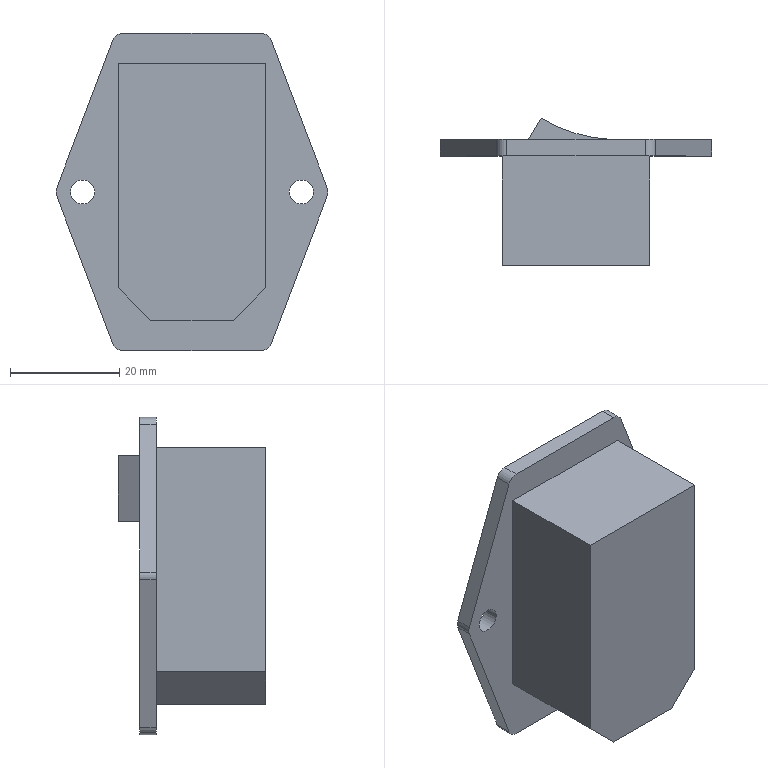Part | STEP file | DIANNAOZIDAIBAOXIANCHAZUO.stp.STEP | 1 solid | 51 faces | box 49.722 x 26.893 x 58 mm | volume 27070 mm3 | plane 40 | cylinder 11 | commonest cylinder face diameters 4 x6 4.4 x4 54.667 x1
STEP:
#1=CARTESIAN_POINT('',(7.5,0.,-23.5));
#2=VERTEX_POINT('',#1);
#3=CARTESIAN_POINT('',(-7.5,0.,-23.5));
#4=VERTEX_POINT('',#3);
#5=CARTESIAN_POINT('',(7.5,0.,-23.5));
#6=DIRECTION('',(-1.,0.,0.));
#7=VECTOR('',#6,1000.);
#8=LINE('',#5,#7);
#9=EDGE_CURVE('',#2,#4,#8,.T.);
#10=ORIENTED_EDGE('',*,*,#9,.F.);
#11=CARTESIAN_POINT('',(13.5,0.,-17.5));
#12=VERTEX_POINT('',#11);
#13=CARTESIAN_POINT('',(13.5,0.,-17.5));
#14=DIRECTION('',(-0.7071,0.,-0.7071));
#15=VECTOR('',#14,1000.);
#16=LINE('',#13,#15);
#17=EDGE_CURVE('',#12,#2,#16,.T.);
#18=ORIENTED_EDGE('',*,*,#17,.F.);
#19=CARTESIAN_POINT('',(13.5,0.,23.5));
#20=VERTEX_POINT('',#19);
#21=CARTESIAN_POINT('',(13.5,0.,23.5));
#22=DIRECTION('',(0.,0.,-1.));
#23=VECTOR('',#22,1000.);
#24=LINE('',#21,#23);
#25=EDGE_CURVE('',#20,#12,#24,.T.);
#26=ORIENTED_EDGE('',*,*,#25,.F.);
#27=CARTESIAN_POINT('',(-13.5,0.,23.5));
#28=VERTEX_POINT('',#27);
#29=CARTESIAN_POINT('',(-13.5,0.,23.5));
#30=DIRECTION('',(1.,0.,0.));
#31=VECTOR('',#30,1000.);
#32=LINE('',#29,#31);
#33=EDGE_CURVE('',#28,#20,#32,.T.);
#34=ORIENTED_EDGE('',*,*,#33,.F.);
#35=CARTESIAN_POINT('',(-13.5,0.,-17.5));
#36=VERTEX_POINT('',#35);
#37=CARTESIAN_POINT('',(-13.5,0.,-17.5));
#38=DIRECTION('',(0.,0.,1.));
#39=VECTOR('',#38,1000.);
#40=LINE('',#37,#39);
#41=EDGE_CURVE('',#36,#28,#40,.T.);
#42=ORIENTED_EDGE('',*,*,#41,.F.);
#43=CARTESIAN_POINT('',(-7.5,0.,-23.5));
#44=DIRECTION('',(-0.7071,0.,0.7071));
#45=VECTOR('',#44,1000.);
#46=LINE('',#43,#45);
#47=EDGE_CURVE('',#4,#36,#46,.T.);
#48=ORIENTED_EDGE('',*,*,#47,.F.);
#49=EDGE_LOOP('',(#10,#18,#26,#34,#42,#48));
#50=FACE_OUTER_BOUND('',#49,.T.);
#51=CARTESIAN_POINT('',(0.,0.,0.));
#52=DIRECTION('',(0.,1.,0.));
#53=DIRECTION('',(1.,0.,0.));
#54=AXIS2_PLACEMENT_3D('',#51,#52,#53);
#55=PLANE('',#54);
#56=ADVANCED_FACE('',(#50),#55,.F.);
#57=CARTESIAN_POINT('',(-7.5,20.,-23.5));
#58=VERTEX_POINT('',#57);
#59=CARTESIAN_POINT('',(-7.5,0.,-23.5));
#60=DIRECTION('',(0.,1.,0.));
#61=VECTOR('',#60,1000.);
#62=LINE('',#59,#61);
#63=EDGE_CURVE('',#4,#58,#62,.T.);
#64=ORIENTED_EDGE('',*,*,#63,.F.);
#65=ORIENTED_EDGE('',*,*,#47,.T.);
#66=CARTESIAN_POINT('',(-13.5,20.,-17.5));
#67=VERTEX_POINT('',#66);
#68=CARTESIAN_POINT('',(-13.5,0.,-17.5));
#69=DIRECTION('',(0.,1.,0.));
#70=VECTOR('',#69,1000.);
#71=LINE('',#68,#70);
#72=EDGE_CURVE('',#36,#67,#71,.T.);
#73=ORIENTED_EDGE('',*,*,#72,.T.);
#74=CARTESIAN_POINT('',(-7.5,20.,-23.5));
#75=DIRECTION('',(-0.7071,0.,0.7071));
#76=VECTOR('',#75,1000.);
#77=LINE('',#74,#76);
#78=EDGE_CURVE('',#58,#67,#77,.T.);
#79=ORIENTED_EDGE('',*,*,#78,.F.);
#80=EDGE_LOOP('',(#64,#65,#73,#79));
#81=FACE_OUTER_BOUND('',#80,.T.);
#82=CARTESIAN_POINT('',(-7.5,0.,-23.5));
#83=DIRECTION('',(-0.7071,0.,-0.7071));
#84=DIRECTION('',(-0.7071,0.,0.7071));
#85=AXIS2_PLACEMENT_3D('',#82,#83,#84);
#86=PLANE('',#85);
#87=ADVANCED_FACE('',(#81),#86,.T.);
#88=CARTESIAN_POINT('',(17.8,20.,0.));
#89=VERTEX_POINT('',#88);
#90=CARTESIAN_POINT('',(22.2,20.,0.));
#91=VERTEX_POINT('',#90);
#92=CARTESIAN_POINT('',(20.,20.,0.));
#93=DIRECTION('',(0.,1.,0.));
#94=DIRECTION('',(-1.,0.,0.));
#95=AXIS2_PLACEMENT_3D('',#92,#93,#94);
#96=CIRCLE('',#95,2.2);
#97=EDGE_CURVE('',#89,#91,#96,.T.);
#98=ORIENTED_EDGE('',*,*,#97,.T.);
#99=CARTESIAN_POINT('',(20.,20.,0.));
#100=DIRECTION('',(0.,1.,0.));
#101=DIRECTION('',(1.,0.,0.));
#102=AXIS2_PLACEMENT_3D('',#99,#100,#101);
#103=CIRCLE('',#102,2.2);
#104=EDGE_CURVE('',#91,#89,#103,.T.);
#105=ORIENTED_EDGE('',*,*,#104,.T.);
#106=EDGE_LOOP('',(#98,#105));
#107=FACE_BOUND('',#106,.T.);
#108=CARTESIAN_POINT('',(-22.2,20.,0.));
#109=VERTEX_POINT('',#108);
#110=CARTESIAN_POINT('',(-17.8,20.,0.));
#111=VERTEX_POINT('',#110);
#112=CARTESIAN_POINT('',(-20.,20.,0.));
#113=DIRECTION('',(0.,1.,0.));
#114=DIRECTION('',(-1.,0.,0.));
#115=AXIS2_PLACEMENT_3D('',#112,#113,#114);
#116=CIRCLE('',#115,2.2);
#117=EDGE_CURVE('',#109,#111,#116,.T.);
#118=ORIENTED_EDGE('',*,*,#117,.T.);
#119=CARTESIAN_POINT('',(-20.,20.,0.));
#120=DIRECTION('',(0.,1.,0.));
#121=DIRECTION('',(1.,0.,0.));
#122=AXIS2_PLACEMENT_3D('',#119,#120,#121);
#123=CIRCLE('',#122,2.2);
#124=EDGE_CURVE('',#111,#109,#123,.T.);
#125=ORIENTED_EDGE('',*,*,#124,.T.);
#126=EDGE_LOOP('',(#118,#125));
#127=FACE_BOUND('',#126,.T.);
#128=CARTESIAN_POINT('',(-13.5,20.,23.5));
#129=VERTEX_POINT('',#128);
#130=CARTESIAN_POINT('',(-13.5,20.,-17.5));
#131=DIRECTION('',(0.,0.,1.));
#132=VECTOR('',#131,1000.);
#133=LINE('',#130,#132);
#134=EDGE_CURVE('',#67,#129,#133,.T.);
#135=ORIENTED_EDGE('',*,*,#134,.T.);
#136=CARTESIAN_POINT('',(13.5,20.,23.5));
#137=VERTEX_POINT('',#136);
#138=CARTESIAN_POINT('',(-13.5,20.,23.5));
#139=DIRECTION('',(1.,0.,0.));
#140=VECTOR('',#139,1000.);
#141=LINE('',#138,#140);
#142=EDGE_CURVE('',#129,#137,#141,.T.);
#143=ORIENTED_EDGE('',*,*,#142,.T.);
#144=CARTESIAN_POINT('',(13.5,20.,-17.5));
#145=VERTEX_POINT('',#144);
#146=CARTESIAN_POINT('',(13.5,20.,23.5));
#147=DIRECTION('',(0.,0.,-1.));
#148=VECTOR('',#147,1000.);
#149=LINE('',#146,#148);
#150=EDGE_CURVE('',#137,#145,#149,.T.);
#151=ORIENTED_EDGE('',*,*,#150,.T.);
#152=CARTESIAN_POINT('',(7.5,20.,-23.5));
#153=VERTEX_POINT('',#152);
#154=CARTESIAN_POINT('',(13.5,20.,-17.5));
#155=DIRECTION('',(-0.7071,0.,-0.7071));
#156=VECTOR('',#155,1000.);
#157=LINE('',#154,#156);
#158=EDGE_CURVE('',#145,#153,#157,.T.);
#159=ORIENTED_EDGE('',*,*,#158,.T.);
#160=CARTESIAN_POINT('',(7.5,20.,-23.5));
#161=DIRECTION('',(-1.,0.,0.));
#162=VECTOR('',#161,1000.);
#163=LINE('',#160,#162);
#164=EDGE_CURVE('',#153,#58,#163,.T.);
#165=ORIENTED_EDGE('',*,*,#164,.T.);
#166=ORIENTED_EDGE('',*,*,#78,.T.);
#167=EDGE_LOOP('',(#135,#143,#151,#159,#165,#166));
#168=FACE_BOUND('',#167,.T.);
#169=CARTESIAN_POINT('',(24.731,20.,-0.7093));
#170=VERTEX_POINT('',#169);
#171=CARTESIAN_POINT('',(14.49,20.,-27.709));
#172=VERTEX_POINT('',#171);
#173=CARTESIAN_POINT('',(24.731,20.,-0.7093));
#174=DIRECTION('',(-0.3547,0.,-0.935));
#175=VECTOR('',#174,1000.);
#176=LINE('',#173,#175);
#177=EDGE_CURVE('',#170,#172,#176,.T.);
#178=ORIENTED_EDGE('',*,*,#177,.F.);
#179=CARTESIAN_POINT('',(24.731,20.,0.7093));
#180=VERTEX_POINT('',#179);
#181=CARTESIAN_POINT('',(22.861,20.,0.));
#182=DIRECTION('',(0.,-1.,0.));
#183=DIRECTION('',(0.935,0.,-0.3547));
#184=AXIS2_PLACEMENT_3D('',#181,#182,#183);
#185=CIRCLE('',#184,2.);
#186=EDGE_CURVE('',#170,#180,#185,.T.);
#187=ORIENTED_EDGE('',*,*,#186,.T.);
#188=CARTESIAN_POINT('',(14.49,20.,27.709));
#189=VERTEX_POINT('',#188);
#190=CARTESIAN_POINT('',(14.49,20.,27.709));
#191=DIRECTION('',(0.3547,0.,-0.935));
#192=VECTOR('',#191,1000.);
#193=LINE('',#190,#192);
#194=EDGE_CURVE('',#189,#180,#193,.T.);
#195=ORIENTED_EDGE('',*,*,#194,.F.);
#196=CARTESIAN_POINT('',(12.62,20.,29.));
#197=VERTEX_POINT('',#196);
#198=CARTESIAN_POINT('',(12.62,20.,27.));
#199=DIRECTION('',(0.,-1.,0.));
#200=DIRECTION('',(0.935,0.,0.3547));
#201=AXIS2_PLACEMENT_3D('',#198,#199,#200);
#202=CIRCLE('',#201,2.);
#203=EDGE_CURVE('',#189,#197,#202,.T.);
#204=ORIENTED_EDGE('',*,*,#203,.T.);
#205=CARTESIAN_POINT('',(-12.62,20.,29.));
#206=VERTEX_POINT('',#205);
#207=CARTESIAN_POINT('',(-12.62,20.,29.));
#208=DIRECTION('',(1.,0.,0.));
#209=VECTOR('',#208,1000.);
#210=LINE('',#207,#209);
#211=EDGE_CURVE('',#206,#197,#210,.T.);
#212=ORIENTED_EDGE('',*,*,#211,.F.);
#213=CARTESIAN_POINT('',(-14.49,20.,27.709));
#214=VERTEX_POINT('',#213);
#215=CARTESIAN_POINT('',(-12.62,20.,27.));
#216=DIRECTION('',(0.,-1.,0.));
#217=DIRECTION('',(0.,0.,1.));
#218=AXIS2_PLACEMENT_3D('',#215,#216,#217);
#219=CIRCLE('',#218,2.);
#220=EDGE_CURVE('',#206,#214,#219,.T.);
#221=ORIENTED_EDGE('',*,*,#220,.T.);
#222=CARTESIAN_POINT('',(-24.731,20.,0.7093));
#223=VERTEX_POINT('',#222);
#224=CARTESIAN_POINT('',(-24.731,20.,0.7093));
#225=DIRECTION('',(0.3547,0.,0.935));
#226=VECTOR('',#225,1000.);
#227=LINE('',#224,#226);
#228=EDGE_CURVE('',#223,#214,#227,.T.);
#229=ORIENTED_EDGE('',*,*,#228,.F.);
#230=CARTESIAN_POINT('',(-24.731,20.,-0.7093));
#231=VERTEX_POINT('',#230);
#232=CARTESIAN_POINT('',(-22.861,20.,0.));
#233=DIRECTION('',(0.,-1.,0.));
#234=DIRECTION('',(-0.935,0.,0.3547));
#235=AXIS2_PLACEMENT_3D('',#232,#233,#234);
#236=CIRCLE('',#235,2.);
#237=EDGE_CURVE('',#223,#231,#236,.T.);
#238=ORIENTED_EDGE('',*,*,#237,.T.);
#239=CARTESIAN_POINT('',(-14.49,20.,-27.709));
#240=VERTEX_POINT('',#239);
#241=CARTESIAN_POINT('',(-14.49,20.,-27.709));
#242=DIRECTION('',(-0.3547,0.,0.935));
#243=VECTOR('',#242,1000.);
#244=LINE('',#241,#243);
#245=EDGE_CURVE('',#240,#231,#244,.T.);
#246=ORIENTED_EDGE('',*,*,#245,.F.);
#247=CARTESIAN_POINT('',(-12.62,20.,-29.));
#248=VERTEX_POINT('',#247);
#249=CARTESIAN_POINT('',(-12.62,20.,-27.));
#250=DIRECTION('',(0.,-1.,0.));
#251=DIRECTION('',(-0.935,0.,-0.3547));
#252=AXIS2_PLACEMENT_3D('',#249,#250,#251);
#253=CIRCLE('',#252,2.);
#254=EDGE_CURVE('',#240,#248,#253,.T.);
#255=ORIENTED_EDGE('',*,*,#254,.T.);
#256=CARTESIAN_POINT('',(12.62,20.,-29.));
#257=VERTEX_POINT('',#256);
#258=CARTESIAN_POINT('',(12.62,20.,-29.));
#259=DIRECTION('',(-1.,0.,0.));
#260=VECTOR('',#259,1000.);
#261=LINE('',#258,#260);
#262=EDGE_CURVE('',#257,#248,#261,.T.);
#263=ORIENTED_EDGE('',*,*,#262,.F.);
#264=CARTESIAN_POINT('',(12.62,20.,-27.));
#265=DIRECTION('',(0.,-1.,0.));
#266=DIRECTION('',(0.,0.,-1.));
#267=AXIS2_PLACEMENT_3D('',#264,#265,#266);
#268=CIRCLE('',#267,2.);
#269=EDGE_CURVE('',#257,#172,#268,.T.);
#270=ORIENTED_EDGE('',*,*,#269,.T.);
#271=EDGE_LOOP('',(#178,#187,#195,#204,#212,#221,#229,#238,#246,#255,#263,#270));
#272=FACE_OUTER_BOUND('',#271,.T.);
#273=CARTESIAN_POINT('',(0.,20.,0.));
#274=DIRECTION('',(0.,1.,0.));
#275=DIRECTION('',(1.,0.,0.));
#276=AXIS2_PLACEMENT_3D('',#273,#274,#275);
#277=PLANE('',#276);
#278=ADVANCED_FACE('',(#107,#127,#168,#272),#277,.F.);
#279=CARTESIAN_POINT('',(7.5,0.,-23.5));
#280=DIRECTION('',(0.,1.,0.));
#281=VECTOR('',#280,1000.);
#282=LINE('',#279,#281);
#283=EDGE_CURVE('',#2,#153,#282,.T.);
#284=ORIENTED_EDGE('',*,*,#283,.F.);
#285=ORIENTED_EDGE('',*,*,#9,.T.);
#286=ORIENTED_EDGE('',*,*,#63,.T.);
#287=ORIENTED_EDGE('',*,*,#164,.F.);
#288=EDGE_LOOP('',(#284,#285,#286,#287));
#289=FACE_OUTER_BOUND('',#288,.T.);
#290=CARTESIAN_POINT('',(7.5,0.,-23.5));
#291=DIRECTION('',(0.,0.,-1.));
#292=DIRECTION('',(0.,-1.,0.));
#293=AXIS2_PLACEMENT_3D('',#290,#291,#292);
#294=PLANE('',#293);
#295=ADVANCED_FACE('',(#289),#294,.T.);
#296=CARTESIAN_POINT('',(13.5,0.,-17.5));
#297=DIRECTION('',(0.,1.,0.));
#298=VECTOR('',#297,1000.);
#299=LINE('',#296,#298);
#300=EDGE_CURVE('',#12,#145,#299,.T.);
#301=ORIENTED_EDGE('',*,*,#300,.F.);
#302=ORIENTED_EDGE('',*,*,#17,.T.);
#303=ORIENTED_EDGE('',*,*,#283,.T.);
#304=ORIENTED_EDGE('',*,*,#158,.F.);
#305=EDGE_LOOP('',(#301,#302,#303,#304));
#306=FACE_OUTER_BOUND('',#305,.T.);
#307=CARTESIAN_POINT('',(13.5,0.,-17.5));
#308=DIRECTION('',(0.7071,0.,-0.7071));
#309=DIRECTION('',(0.,-1.,0.));
#310=AXIS2_PLACEMENT_3D('',#307,#308,#309);
#311=PLANE('',#310);
#312=ADVANCED_FACE('',(#306),#311,.T.);
#313=CARTESIAN_POINT('',(13.5,0.,23.5));
#314=DIRECTION('',(0.,1.,0.));
#315=VECTOR('',#314,1000.);
#316=LINE('',#313,#315);
#317=EDGE_CURVE('',#20,#137,#316,.T.);
#318=ORIENTED_EDGE('',*,*,#317,.F.);
#319=ORIENTED_EDGE('',*,*,#25,.T.);
#320=ORIENTED_EDGE('',*,*,#300,.T.);
#321=ORIENTED_EDGE('',*,*,#150,.F.);
#322=EDGE_LOOP('',(#318,#319,#320,#321));
#323=FACE_OUTER_BOUND('',#322,.T.);
#324=CARTESIAN_POINT('',(13.5,0.,23.5));
#325=DIRECTION('',(1.,0.,0.));
#326=DIRECTION('',(0.,1.,0.));
#327=AXIS2_PLACEMENT_3D('',#324,#325,#326);
#328=PLANE('',#327);
#329=ADVANCED_FACE('',(#323),#328,.T.);
#330=CARTESIAN_POINT('',(-13.5,0.,23.5));
#331=DIRECTION('',(0.,1.,0.));
#332=VECTOR('',#331,1000.);
#333=LINE('',#330,#332);
#334=EDGE_CURVE('',#28,#129,#333,.T.);
#335=ORIENTED_EDGE('',*,*,#334,.F.);
#336=ORIENTED_EDGE('',*,*,#33,.T.);
#337=ORIENTED_EDGE('',*,*,#317,.T.);
#338=ORIENTED_EDGE('',*,*,#142,.F.);
#339=EDGE_LOOP('',(#335,#336,#337,#338));
#340=FACE_OUTER_BOUND('',#339,.T.);
#341=CARTESIAN_POINT('',(-13.5,0.,23.5));
#342=DIRECTION('',(0.,0.,1.));
#343=DIRECTION('',(1.,0.,0.));
#344=AXIS2_PLACEMENT_3D('',#341,#342,#343);
#345=PLANE('',#344);
#346=ADVANCED_FACE('',(#340),#345,.T.);
#347=ORIENTED_EDGE('',*,*,#72,.F.);
#348=ORIENTED_EDGE('',*,*,#41,.T.);
#349=ORIENTED_EDGE('',*,*,#334,.T.);
#350=ORIENTED_EDGE('',*,*,#134,.F.);
#351=EDGE_LOOP('',(#347,#348,#349,#350));
#352=FACE_OUTER_BOUND('',#351,.T.);
#353=CARTESIAN_POINT('',(-13.5,0.,-17.5));
#354=DIRECTION('',(-1.,0.,0.));
#355=DIRECTION('',(0.,0.,1.));
#356=AXIS2_PLACEMENT_3D('',#353,#354,#355);
#357=PLANE('',#356);
#358=ADVANCED_FACE('',(#352),#357,.T.);
#359=CARTESIAN_POINT('',(22.2,23.,0.));
#360=VERTEX_POINT('',#359);
#361=CARTESIAN_POINT('',(22.2,23.,0.));
#362=DIRECTION('',(0.,-1.,0.));
#363=VECTOR('',#362,1000.);
#364=LINE('',#361,#363);
#365=EDGE_CURVE('',#360,#91,#364,.T.);
#366=ORIENTED_EDGE('',*,*,#365,.F.);
#367=CARTESIAN_POINT('',(17.8,23.,0.));
#368=VERTEX_POINT('',#367);
#369=CARTESIAN_POINT('',(20.,23.,0.));
#370=DIRECTION('',(0.,1.,0.));
#371=DIRECTION('',(1.,0.,0.));
#372=AXIS2_PLACEMENT_3D('',#369,#370,#371);
#373=CIRCLE('',#372,2.2);
#374=EDGE_CURVE('',#360,#368,#373,.T.);
#375=ORIENTED_EDGE('',*,*,#374,.T.);
#376=CARTESIAN_POINT('',(17.8,23.,0.));
#377=DIRECTION('',(0.,-1.,0.));
#378=VECTOR('',#377,1000.);
#379=LINE('',#376,#378);
#380=EDGE_CURVE('',#368,#89,#379,.T.);
#381=ORIENTED_EDGE('',*,*,#380,.T.);
#382=ORIENTED_EDGE('',*,*,#104,.F.);
#383=EDGE_LOOP('',(#366,#375,#381,#382));
#384=FACE_OUTER_BOUND('',#383,.T.);
#385=CARTESIAN_POINT('',(20.,23.,0.));
#386=DIRECTION('',(0.,1.,0.));
#387=DIRECTION('',(1.,0.,0.));
#388=AXIS2_PLACEMENT_3D('',#385,#386,#387);
#389=CYLINDRICAL_SURFACE('',#388,2.2);
#390=ADVANCED_FACE('',(#384),#389,.F.);
#391=ORIENTED_EDGE('',*,*,#380,.F.);
#392=CARTESIAN_POINT('',(20.,23.,0.));
#393=DIRECTION('',(0.,1.,0.));
#394=DIRECTION('',(-1.,0.,0.));
#395=AXIS2_PLACEMENT_3D('',#392,#393,#394);
#396=CIRCLE('',#395,2.2);
#397=EDGE_CURVE('',#368,#360,#396,.T.);
#398=ORIENTED_EDGE('',*,*,#397,.T.);
#399=ORIENTED_EDGE('',*,*,#365,.T.);
#400=ORIENTED_EDGE('',*,*,#97,.F.);
#401=EDGE_LOOP('',(#391,#398,#399,#400));
#402=FACE_OUTER_BOUND('',#401,.T.);
#403=CARTESIAN_POINT('',(20.,23.,0.));
#404=DIRECTION('',(0.,1.,0.));
#405=DIRECTION('',(1.,0.,0.));
#406=AXIS2_PLACEMENT_3D('',#403,#404,#405);
#407=CYLINDRICAL_SURFACE('',#406,2.2);
#408=ADVANCED_FACE('',(#402),#407,.F.);
#409=CARTESIAN_POINT('',(-22.2,23.,0.));
#410=VERTEX_POINT('',#409);
#411=CARTESIAN_POINT('',(-17.8,23.,0.));
#412=VERTEX_POINT('',#411);
#413=CARTESIAN_POINT('',(-20.,23.,0.));
#414=DIRECTION('',(0.,1.,0.));
#415=DIRECTION('',(-1.,0.,0.));
#416=AXIS2_PLACEMENT_3D('',#413,#414,#415);
#417=CIRCLE('',#416,2.2);
#418=EDGE_CURVE('',#410,#412,#417,.T.);
#419=ORIENTED_EDGE('',*,*,#418,.F.);
#420=CARTESIAN_POINT('',(-20.,23.,0.));
#421=DIRECTION('',(0.,1.,0.));
#422=DIRECTION('',(1.,0.,0.));
#423=AXIS2_PLACEMENT_3D('',#420,#421,#422);
#424=CIRCLE('',#423,2.2);
#425=EDGE_CURVE('',#412,#410,#424,.T.);
#426=ORIENTED_EDGE('',*,*,#425,.F.);
#427=EDGE_LOOP('',(#419,#426));
#428=FACE_BOUND('',#427,.T.);
#429=ORIENTED_EDGE('',*,*,#397,.F.);
#430=ORIENTED_EDGE('',*,*,#374,.F.);
#431=EDGE_LOOP('',(#429,#430));
#432=FACE_BOUND('',#431,.T.);
#433=CARTESIAN_POINT('',(7.5,23.,-23.));
#434=VERTEX_POINT('',#433);
#435=CARTESIAN_POINT('',(-7.5,23.,-23.));
#436=VERTEX_POINT('',#435);
#437=CARTESIAN_POINT('',(7.5,23.,-23.));
#438=DIRECTION('',(-1.,0.,0.));
#439=VECTOR('',#438,1000.);
#440=LINE('',#437,#439);
#441=EDGE_CURVE('',#434,#436,#440,.T.);
#442=ORIENTED_EDGE('',*,*,#441,.F.);
#443=CARTESIAN_POINT('',(12.,23.,-18.5));
#444=VERTEX_POINT('',#443);
#445=CARTESIAN_POINT('',(12.,23.,-18.5));
#446=DIRECTION('',(-0.7071,0.,-0.7071));
#447=VECTOR('',#446,1000.);
#448=LINE('',#445,#447);
#449=EDGE_CURVE('',#444,#434,#448,.T.);
#450=ORIENTED_EDGE('',*,*,#449,.F.);
#451=CARTESIAN_POINT('',(12.,23.,-6.));
#452=VERTEX_POINT('',#451);
#453=CARTESIAN_POINT('',(12.,23.,-6.));
#454=DIRECTION('',(0.,0.,-1.));
#455=VECTOR('',#454,1000.);
#456=LINE('',#453,#455);
#457=EDGE_CURVE('',#452,#444,#456,.T.);
#458=ORIENTED_EDGE('',*,*,#457,.F.);
#459=CARTESIAN_POINT('',(-12.,23.,-6.));
#460=VERTEX_POINT('',#459);
#461=CARTESIAN_POINT('',(-12.,23.,-6.));
#462=DIRECTION('',(1.,0.,0.));
#463=VECTOR('',#462,1000.);
#464=LINE('',#461,#463);
#465=EDGE_CURVE('',#460,#452,#464,.T.);
#466=ORIENTED_EDGE('',*,*,#465,.F.);
#467=CARTESIAN_POINT('',(-12.,23.,-18.5));
#468=VERTEX_POINT('',#467);
#469=CARTESIAN_POINT('',(-12.,23.,-18.5));
#470=DIRECTION('',(0.,0.,1.));
#471=VECTOR('',#470,1000.);
#472=LINE('',#469,#471);
#473=EDGE_CURVE('',#468,#460,#472,.T.);
#474=ORIENTED_EDGE('',*,*,#473,.F.);
#475=CARTESIAN_POINT('',(-7.5,23.,-23.));
#476=DIRECTION('',(-0.7071,0.,0.7071));
#477=VECTOR('',#476,1000.);
#478=LINE('',#475,#477);
#479=EDGE_CURVE('',#436,#468,#478,.T.);
#480=ORIENTED_EDGE('',*,*,#479,.F.);
#481=EDGE_LOOP('',(#442,#450,#458,#466,#474,#480));
#482=FACE_BOUND('',#481,.T.);
#483=CARTESIAN_POINT('',(6.51,23.,10.));
#484=VERTEX_POINT('',#483);
#485=CARTESIAN_POINT('',(6.51,23.,22.));
#486=VERTEX_POINT('',#485);
#487=CARTESIAN_POINT('',(6.51,23.,10.));
#488=DIRECTION('',(0.,0.,1.));
#489=VECTOR('',#488,1000.);
#490=LINE('',#487,#489);
#491=EDGE_CURVE('',#484,#486,#490,.T.);
#492=ORIENTED_EDGE('',*,*,#491,.T.);
#493=CARTESIAN_POINT('',(-8.737,23.,22.));
#494=VERTEX_POINT('',#493);
#495=CARTESIAN_POINT('',(-8.737,23.,22.));
#496=DIRECTION('',(1.,0.,0.));
#497=VECTOR('',#496,1000.);
#498=LINE('',#495,#497);
#499=EDGE_CURVE('',#494,#486,#498,.T.);
#500=ORIENTED_EDGE('',*,*,#499,.F.);
#501=CARTESIAN_POINT('',(-8.737,23.,10.));
#502=VERTEX_POINT('',#501);
#503=CARTESIAN_POINT('',(-8.737,23.,10.));
#504=DIRECTION('',(0.,0.,1.));
#505=VECTOR('',#504,1000.);
#506=LINE('',#503,#505);
#507=EDGE_CURVE('',#502,#494,#506,.T.);
#508=ORIENTED_EDGE('',*,*,#507,.F.);
#509=CARTESIAN_POINT('',(-8.737,23.,10.));
#510=DIRECTION('',(1.,0.,0.));
#511=VECTOR('',#510,1000.);
#512=LINE('',#509,#511);
#513=EDGE_CURVE('',#502,#484,#512,.T.);
#514=ORIENTED_EDGE('',*,*,#513,.T.);
#515=EDGE_LOOP('',(#492,#500,#508,#514));
#516=FACE_BOUND('',#515,.T.);
#517=CARTESIAN_POINT('',(12.62,23.,-29.));
#518=VERTEX_POINT('',#517);
#519=CARTESIAN_POINT('',(-12.62,23.,-29.));
#520=VERTEX_POINT('',#519);
#521=CARTESIAN_POINT('',(12.62,23.,-29.));
#522=DIRECTION('',(-1.,0.,0.));
#523=VECTOR('',#522,1000.);
#524=LINE('',#521,#523);
#525=EDGE_CURVE('',#518,#520,#524,.T.);
#526=ORIENTED_EDGE('',*,*,#525,.T.);
#527=CARTESIAN_POINT('',(-14.49,23.,-27.709));
#528=VERTEX_POINT('',#527);
#529=CARTESIAN_POINT('',(-12.62,23.,-27.));
#530=DIRECTION('',(0.,1.,0.));
#531=DIRECTION('',(0.,0.,-1.));
#532=AXIS2_PLACEMENT_3D('',#529,#530,#531);
#533=CIRCLE('',#532,2.);
#534=EDGE_CURVE('',#520,#528,#533,.T.);
#535=ORIENTED_EDGE('',*,*,#534,.T.);
#536=CARTESIAN_POINT('',(-24.731,23.,-0.7093));
#537=VERTEX_POINT('',#536);
#538=CARTESIAN_POINT('',(-14.49,23.,-27.709));
#539=DIRECTION('',(-0.3547,0.,0.935));
#540=VECTOR('',#539,1000.);
#541=LINE('',#538,#540);
#542=EDGE_CURVE('',#528,#537,#541,.T.);
#543=ORIENTED_EDGE('',*,*,#542,.T.);
#544=CARTESIAN_POINT('',(-24.731,23.,0.7093));
#545=VERTEX_POINT('',#544);
#546=CARTESIAN_POINT('',(-22.861,23.,0.));
#547=DIRECTION('',(0.,1.,0.));
#548=DIRECTION('',(-0.935,0.,-0.3547));
#549=AXIS2_PLACEMENT_3D('',#546,#547,#548);
#550=CIRCLE('',#549,2.);
#551=EDGE_CURVE('',#537,#545,#550,.T.);
#552=ORIENTED_EDGE('',*,*,#551,.T.);
#553=CARTESIAN_POINT('',(-14.49,23.,27.709));
#554=VERTEX_POINT('',#553);
#555=CARTESIAN_POINT('',(-24.731,23.,0.7093));
#556=DIRECTION('',(0.3547,0.,0.935));
#557=VECTOR('',#556,1000.);
#558=LINE('',#555,#557);
#559=EDGE_CURVE('',#545,#554,#558,.T.);
#560=ORIENTED_EDGE('',*,*,#559,.T.);
#561=CARTESIAN_POINT('',(-12.62,23.,29.));
#562=VERTEX_POINT('',#561);
#563=CARTESIAN_POINT('',(-12.62,23.,27.));
#564=DIRECTION('',(0.,1.,0.));
#565=DIRECTION('',(-0.935,0.,0.3547));
#566=AXIS2_PLACEMENT_3D('',#563,#564,#565);
#567=CIRCLE('',#566,2.);
#568=EDGE_CURVE('',#554,#562,#567,.T.);
#569=ORIENTED_EDGE('',*,*,#568,.T.);
#570=CARTESIAN_POINT('',(12.62,23.,29.));
#571=VERTEX_POINT('',#570);
#572=CARTESIAN_POINT('',(-12.62,23.,29.));
#573=DIRECTION('',(1.,0.,0.));
#574=VECTOR('',#573,1000.);
#575=LINE('',#572,#574);
#576=EDGE_CURVE('',#562,#571,#575,.T.);
#577=ORIENTED_EDGE('',*,*,#576,.T.);
#578=CARTESIAN_POINT('',(14.49,23.,27.709));
#579=VERTEX_POINT('',#578);
#580=CARTESIAN_POINT('',(12.62,23.,27.));
#581=DIRECTION('',(0.,1.,0.));
#582=DIRECTION('',(0.,0.,1.));
#583=AXIS2_PLACEMENT_3D('',#580,#581,#582);
#584=CIRCLE('',#583,2.);
#585=EDGE_CURVE('',#571,#579,#584,.T.);
#586=ORIENTED_EDGE('',*,*,#585,.T.);
#587=CARTESIAN_POINT('',(24.731,23.,0.7093));
#588=VERTEX_POINT('',#587);
#589=CARTESIAN_POINT('',(14.49,23.,27.709));
#590=DIRECTION('',(0.3547,0.,-0.935));
#591=VECTOR('',#590,1000.);
#592=LINE('',#589,#591);
#593=EDGE_CURVE('',#579,#588,#592,.T.);
#594=ORIENTED_EDGE('',*,*,#593,.T.);
#595=CARTESIAN_POINT('',(24.731,23.,-0.7093));
#596=VERTEX_POINT('',#595);
#597=CARTESIAN_POINT('',(22.861,23.,0.));
#598=DIRECTION('',(0.,1.,0.));
#599=DIRECTION('',(0.935,0.,0.3547));
#600=AXIS2_PLACEMENT_3D('',#597,#598,#599);
#601=CIRCLE('',#600,2.);
#602=EDGE_CURVE('',#588,#596,#601,.T.);
#603=ORIENTED_EDGE('',*,*,#602,.T.);
#604=CARTESIAN_POINT('',(14.49,23.,-27.709));
#605=VERTEX_POINT('',#604);
#606=CARTESIAN_POINT('',(24.731,23.,-0.7093));
#607=DIRECTION('',(-0.3547,0.,-0.935));
#608=VECTOR('',#607,1000.);
#609=LINE('',#606,#608);
#610=EDGE_CURVE('',#596,#605,#609,.T.);
#611=ORIENTED_EDGE('',*,*,#610,.T.);
#612=CARTESIAN_POINT('',(12.62,23.,-27.));
#613=DIRECTION('',(0.,1.,0.));
#614=DIRECTION('',(0.935,0.,-0.3547));
#615=AXIS2_PLACEMENT_3D('',#612,#613,#614);
#616=CIRCLE('',#615,2.);
#617=EDGE_CURVE('',#605,#518,#616,.T.);
#618=ORIENTED_EDGE('',*,*,#617,.T.);
#619=EDGE_LOOP('',(#526,#535,#543,#552,#560,#569,#577,#586,#594,#603,#611,#618));
#620=FACE_OUTER_BOUND('',#619,.T.);
#621=CARTESIAN_POINT('',(0.,23.,0.));
#622=DIRECTION('',(0.,1.,0.));
#623=DIRECTION('',(1.,0.,0.));
#624=AXIS2_PLACEMENT_3D('',#621,#622,#623);
#625=PLANE('',#624);
#626=ADVANCED_FACE('',(#428,#432,#482,#516,#620),#625,.T.);
#627=CARTESIAN_POINT('',(-17.8,23.,0.));
#628=DIRECTION('',(0.,-1.,0.));
#629=VECTOR('',#628,1000.);
#630=LINE('',#627,#629);
#631=EDGE_CURVE('',#412,#111,#630,.T.);
#632=ORIENTED_EDGE('',*,*,#631,.F.);
#633=ORIENTED_EDGE('',*,*,#425,.T.);
#634=CARTESIAN_POINT('',(-22.2,23.,0.));
#635=DIRECTION('',(0.,-1.,0.));
#636=VECTOR('',#635,1000.);
#637=LINE('',#634,#636);
#638=EDGE_CURVE('',#410,#109,#637,.T.);
#639=ORIENTED_EDGE('',*,*,#638,.T.);
#640=ORIENTED_EDGE('',*,*,#124,.F.);
#641=EDGE_LOOP('',(#632,#633,#639,#640));
#642=FACE_OUTER_BOUND('',#641,.T.);
#643=CARTESIAN_POINT('',(-20.,23.,0.));
#644=DIRECTION('',(0.,1.,0.));
#645=DIRECTION('',(1.,0.,0.));
#646=AXIS2_PLACEMENT_3D('',#643,#644,#645);
#647=CYLINDRICAL_SURFACE('',#646,2.2);
#648=ADVANCED_FACE('',(#642),#647,.F.);
#649=ORIENTED_EDGE('',*,*,#638,.F.);
#650=ORIENTED_EDGE('',*,*,#418,.T.);
#651=ORIENTED_EDGE('',*,*,#631,.T.);
#652=ORIENTED_EDGE('',*,*,#117,.F.);
#653=EDGE_LOOP('',(#649,#650,#651,#652));
#654=FACE_OUTER_BOUND('',#653,.T.);
#655=CARTESIAN_POINT('',(-20.,23.,0.));
#656=DIRECTION('',(0.,1.,0.));
#657=DIRECTION('',(1.,0.,0.));
#658=AXIS2_PLACEMENT_3D('',#655,#656,#657);
#659=CYLINDRICAL_SURFACE('',#658,2.2);
#660=ADVANCED_FACE('',(#654),#659,.F.);
#661=CARTESIAN_POINT('',(12.62,23.,-29.));
#662=DIRECTION('',(0.,-1.,0.));
#663=VECTOR('',#662,1000.);
#664=LINE('',#661,#663);
#665=EDGE_CURVE('',#518,#257,#664,.T.);
#666=ORIENTED_EDGE('',*,*,#665,.F.);
#667=ORIENTED_EDGE('',*,*,#617,.F.);
#668=CARTESIAN_POINT('',(14.49,23.,-27.709));
#669=DIRECTION('',(0.,-1.,0.));
#670=VECTOR('',#669,1000.);
#671=LINE('',#668,#670);
#672=EDGE_CURVE('',#605,#172,#671,.T.);
#673=ORIENTED_EDGE('',*,*,#672,.T.);
#674=ORIENTED_EDGE('',*,*,#269,.F.);
#675=EDGE_LOOP('',(#666,#667,#673,#674));
#676=FACE_OUTER_BOUND('',#675,.T.);
#677=CARTESIAN_POINT('',(12.62,52.983,-27.));
#678=DIRECTION('',(0.,-1.,0.));
#679=DIRECTION('',(0.,0.,-1.));
#680=AXIS2_PLACEMENT_3D('',#677,#678,#679);
#681=CYLINDRICAL_SURFACE('',#680,2.);
#682=ADVANCED_FACE('',(#676),#681,.T.);
#683=ORIENTED_EDGE('',*,*,#610,.F.);
#684=CARTESIAN_POINT('',(24.731,23.,-0.7093));
#685=DIRECTION('',(0.,-1.,0.));
#686=VECTOR('',#685,1000.);
#687=LINE('',#684,#686);
#688=EDGE_CURVE('',#596,#170,#687,.T.);
#689=ORIENTED_EDGE('',*,*,#688,.T.);
#690=ORIENTED_EDGE('',*,*,#177,.T.);
#691=ORIENTED_EDGE('',*,*,#672,.F.);
#692=EDGE_LOOP('',(#683,#689,#690,#691));
#693=FACE_OUTER_BOUND('',#692,.T.);
#694=CARTESIAN_POINT('',(25.,20.,0.));
#695=DIRECTION('',(0.935,0.,-0.3547));
#696=DIRECTION('',(0.,-1.,0.));
#697=AXIS2_PLACEMENT_3D('',#694,#695,#696);
#698=PLANE('',#697);
#699=ADVANCED_FACE('',(#693),#698,.T.);
#700=ORIENTED_EDGE('',*,*,#688,.F.);
#701=ORIENTED_EDGE('',*,*,#602,.F.);
#702=CARTESIAN_POINT('',(24.731,23.,0.7093));
#703=DIRECTION('',(0.,-1.,0.));
#704=VECTOR('',#703,1000.);
#705=LINE('',#702,#704);
#706=EDGE_CURVE('',#588,#180,#705,.T.);
#707=ORIENTED_EDGE('',*,*,#706,.T.);
#708=ORIENTED_EDGE('',*,*,#186,.F.);
#709=EDGE_LOOP('',(#700,#701,#707,#708));
#710=FACE_OUTER_BOUND('',#709,.T.);
#711=CARTESIAN_POINT('',(22.861,52.983,0.));
#712=DIRECTION('',(0.,-1.,0.));
#713=DIRECTION('',(0.935,0.,-0.3547));
#714=AXIS2_PLACEMENT_3D('',#711,#712,#713);
#715=CYLINDRICAL_SURFACE('',#714,2.);
#716=ADVANCED_FACE('',(#710),#715,.T.);
#717=ORIENTED_EDGE('',*,*,#194,.T.);
#718=ORIENTED_EDGE('',*,*,#706,.F.);
#719=ORIENTED_EDGE('',*,*,#593,.F.);
#720=CARTESIAN_POINT('',(14.49,23.,27.709));
#721=DIRECTION('',(0.,-1.,0.));
#722=VECTOR('',#721,1000.);
#723=LINE('',#720,#722);
#724=EDGE_CURVE('',#579,#189,#723,.T.);
#725=ORIENTED_EDGE('',*,*,#724,.T.);
#726=EDGE_LOOP('',(#717,#718,#719,#725));
#727=FACE_OUTER_BOUND('',#726,.T.);
#728=CARTESIAN_POINT('',(14.,20.,29.));
#729=DIRECTION('',(0.935,0.,0.3547));
#730=DIRECTION('',(0.,-1.,0.));
#731=AXIS2_PLACEMENT_3D('',#728,#729,#730);
#732=PLANE('',#731);
#733=ADVANCED_FACE('',(#727),#732,.T.);
#734=ORIENTED_EDGE('',*,*,#724,.F.);
#735=ORIENTED_EDGE('',*,*,#585,.F.);
#736=CARTESIAN_POINT('',(12.62,23.,29.));
#737=DIRECTION('',(0.,-1.,0.));
#738=VECTOR('',#737,1000.);
#739=LINE('',#736,#738);
#740=EDGE_CURVE('',#571,#197,#739,.T.);
#741=ORIENTED_EDGE('',*,*,#740,.T.);
#742=ORIENTED_EDGE('',*,*,#203,.F.);
#743=EDGE_LOOP('',(#734,#735,#741,#742));
#744=FACE_OUTER_BOUND('',#743,.T.);
#745=CARTESIAN_POINT('',(12.62,52.983,27.));
#746=DIRECTION('',(0.,-1.,0.));
#747=DIRECTION('',(0.935,0.,0.3547));
#748=AXIS2_PLACEMENT_3D('',#745,#746,#747);
#749=CYLINDRICAL_SURFACE('',#748,2.);
#750=ADVANCED_FACE('',(#744),#749,.T.);
#751=ORIENTED_EDGE('',*,*,#211,.T.);
#752=ORIENTED_EDGE('',*,*,#740,.F.);
#753=ORIENTED_EDGE('',*,*,#576,.F.);
#754=CARTESIAN_POINT('',(-12.62,23.,29.));
#755=DIRECTION('',(0.,-1.,0.));
#756=VECTOR('',#755,1000.);
#757=LINE('',#754,#756);
#758=EDGE_CURVE('',#562,#206,#757,.T.);
#759=ORIENTED_EDGE('',*,*,#758,.T.);
#760=EDGE_LOOP('',(#751,#752,#753,#759));
#761=FACE_OUTER_BOUND('',#760,.T.);
#762=CARTESIAN_POINT('',(-14.,20.,29.));
#763=DIRECTION('',(0.,0.,1.));
#764=DIRECTION('',(1.,0.,0.));
#765=AXIS2_PLACEMENT_3D('',#762,#763,#764);
#766=PLANE('',#765);
#767=ADVANCED_FACE('',(#761),#766,.T.);
#768=ORIENTED_EDGE('',*,*,#758,.F.);
#769=ORIENTED_EDGE('',*,*,#568,.F.);
#770=CARTESIAN_POINT('',(-14.49,23.,27.709));
#771=DIRECTION('',(0.,-1.,0.));
#772=VECTOR('',#771,1000.);
#773=LINE('',#770,#772);
#774=EDGE_CURVE('',#554,#214,#773,.T.);
#775=ORIENTED_EDGE('',*,*,#774,.T.);
#776=ORIENTED_EDGE('',*,*,#220,.F.);
#777=EDGE_LOOP('',(#768,#769,#775,#776));
#778=FACE_OUTER_BOUND('',#777,.T.);
#779=CARTESIAN_POINT('',(-12.62,52.983,27.));
#780=DIRECTION('',(0.,-1.,0.));
#781=DIRECTION('',(0.,0.,1.));
#782=AXIS2_PLACEMENT_3D('',#779,#780,#781);
#783=CYLINDRICAL_SURFACE('',#782,2.);
#784=ADVANCED_FACE('',(#778),#783,.T.);
#785=ORIENTED_EDGE('',*,*,#228,.T.);
#786=ORIENTED_EDGE('',*,*,#774,.F.);
#787=ORIENTED_EDGE('',*,*,#559,.F.);
#788=CARTESIAN_POINT('',(-24.731,23.,0.7093));
#789=DIRECTION('',(0.,-1.,0.));
#790=VECTOR('',#789,1000.);
#791=LINE('',#788,#790);
#792=EDGE_CURVE('',#545,#223,#791,.T.);
#793=ORIENTED_EDGE('',*,*,#792,.T.);
#794=EDGE_LOOP('',(#785,#786,#787,#793));
#795=FACE_OUTER_BOUND('',#794,.T.);
#796=CARTESIAN_POINT('',(-25.,20.,0.));
#797=DIRECTION('',(-0.935,0.,0.3547));
#798=DIRECTION('',(0.,1.,0.));
#799=AXIS2_PLACEMENT_3D('',#796,#797,#798);
#800=PLANE('',#799);
#801=ADVANCED_FACE('',(#795),#800,.T.);
#802=ORIENTED_EDGE('',*,*,#792,.F.);
#803=ORIENTED_EDGE('',*,*,#551,.F.);
#804=CARTESIAN_POINT('',(-24.731,23.,-0.7093));
#805=DIRECTION('',(0.,-1.,0.));
#806=VECTOR('',#805,1000.);
#807=LINE('',#804,#806);
#808=EDGE_CURVE('',#537,#231,#807,.T.);
#809=ORIENTED_EDGE('',*,*,#808,.T.);
#810=ORIENTED_EDGE('',*,*,#237,.F.);
#811=EDGE_LOOP('',(#802,#803,#809,#810));
#812=FACE_OUTER_BOUND('',#811,.T.);
#813=CARTESIAN_POINT('',(-22.861,52.983,0.));
#814=DIRECTION('',(0.,-1.,0.));
#815=DIRECTION('',(-0.935,0.,0.3547));
#816=AXIS2_PLACEMENT_3D('',#813,#814,#815);
#817=CYLINDRICAL_SURFACE('',#816,2.);
#818=ADVANCED_FACE('',(#812),#817,.T.);
#819=ORIENTED_EDGE('',*,*,#245,.T.);
#820=ORIENTED_EDGE('',*,*,#808,.F.);
#821=ORIENTED_EDGE('',*,*,#542,.F.);
#822=CARTESIAN_POINT('',(-14.49,23.,-27.709));
#823=DIRECTION('',(0.,-1.,0.));
#824=VECTOR('',#823,1000.);
#825=LINE('',#822,#824);
#826=EDGE_CURVE('',#528,#240,#825,.T.);
#827=ORIENTED_EDGE('',*,*,#826,.T.);
#828=EDGE_LOOP('',(#819,#820,#821,#827));
#829=FACE_OUTER_BOUND('',#828,.T.);
#830=CARTESIAN_POINT('',(-14.,20.,-29.));
#831=DIRECTION('',(-0.935,0.,-0.3547));
#832=DIRECTION('',(-0.3547,0.,0.935));
#833=AXIS2_PLACEMENT_3D('',#830,#831,#832);
#834=PLANE('',#833);
#835=ADVANCED_FACE('',(#829),#834,.T.);
#836=ORIENTED_EDGE('',*,*,#826,.F.);
#837=ORIENTED_EDGE('',*,*,#534,.F.);
#838=CARTESIAN_POINT('',(-12.62,23.,-29.));
#839=DIRECTION('',(0.,-1.,0.));
#840=VECTOR('',#839,1000.);
#841=LINE('',#838,#840);
#842=EDGE_CURVE('',#520,#248,#841,.T.);
#843=ORIENTED_EDGE('',*,*,#842,.T.);
#844=ORIENTED_EDGE('',*,*,#254,.F.);
#845=EDGE_LOOP('',(#836,#837,#843,#844));
#846=FACE_OUTER_BOUND('',#845,.T.);
#847=CARTESIAN_POINT('',(-12.62,52.983,-27.));
#848=DIRECTION('',(0.,-1.,0.));
#849=DIRECTION('',(-0.935,0.,-0.3547));
#850=AXIS2_PLACEMENT_3D('',#847,#848,#849);
#851=CYLINDRICAL_SURFACE('',#850,2.);
#852=ADVANCED_FACE('',(#846),#851,.T.);
#853=ORIENTED_EDGE('',*,*,#262,.T.);
#854=ORIENTED_EDGE('',*,*,#842,.F.);
#855=ORIENTED_EDGE('',*,*,#525,.F.);
#856=ORIENTED_EDGE('',*,*,#665,.T.);
#857=EDGE_LOOP('',(#853,#854,#855,#856));
#858=FACE_OUTER_BOUND('',#857,.T.);
#859=CARTESIAN_POINT('',(14.,20.,-29.));
#860=DIRECTION('',(0.,0.,-1.));
#861=DIRECTION('',(0.,-1.,0.));
#862=AXIS2_PLACEMENT_3D('',#859,#860,#861);
#863=PLANE('',#862);
#864=ADVANCED_FACE('',(#858),#863,.T.);
#865=CARTESIAN_POINT('',(-12.,11.,-18.5));
#866=VERTEX_POINT('',#865);
#867=CARTESIAN_POINT('',(-12.,23.,-18.5));
#868=DIRECTION('',(0.,-1.,0.));
#869=VECTOR('',#868,1000.);
#870=LINE('',#867,#869);
#871=EDGE_CURVE('',#468,#866,#870,.T.);
#872=ORIENTED_EDGE('',*,*,#871,.T.);
#873=CARTESIAN_POINT('',(-7.5,11.,-23.));
#874=VERTEX_POINT('',#873);
#875=CARTESIAN_POINT('',(-7.5,11.,-23.));
#876=DIRECTION('',(-0.7071,0.,0.7071));
#877=VECTOR('',#876,1000.);
#878=LINE('',#875,#877);
#879=EDGE_CURVE('',#874,#866,#878,.T.);
#880=ORIENTED_EDGE('',*,*,#879,.F.);
#881=CARTESIAN_POINT('',(-7.5,23.,-23.));
#882=DIRECTION('',(0.,-1.,0.));
#883=VECTOR('',#882,1000.);
#884=LINE('',#881,#883);
#885=EDGE_CURVE('',#436,#874,#884,.T.);
#886=ORIENTED_EDGE('',*,*,#885,.F.);
#887=ORIENTED_EDGE('',*,*,#479,.T.);
#888=EDGE_LOOP('',(#872,#880,#886,#887));
#889=FACE_OUTER_BOUND('',#888,.T.);
#890=CARTESIAN_POINT('',(-7.5,23.,-23.));
#891=DIRECTION('',(-0.7071,0.,-0.7071));
#892=DIRECTION('',(-0.7071,0.,0.7071));
#893=AXIS2_PLACEMENT_3D('',#890,#891,#892);
#894=PLANE('',#893);
#895=ADVANCED_FACE('',(#889),#894,.F.);
#896=ORIENTED_EDGE('',*,*,#885,.T.);
#897=CARTESIAN_POINT('',(7.5,11.,-23.));
#898=VERTEX_POINT('',#897);
#899=CARTESIAN_POINT('',(7.5,11.,-23.));
#900=DIRECTION('',(-1.,0.,0.));
#901=VECTOR('',#900,1000.);
#902=LINE('',#899,#901);
#903=EDGE_CURVE('',#898,#874,#902,.T.);
#904=ORIENTED_EDGE('',*,*,#903,.F.);
#905=CARTESIAN_POINT('',(7.5,23.,-23.));
#906=DIRECTION('',(0.,-1.,0.));
#907=VECTOR('',#906,1000.);
#908=LINE('',#905,#907);
#909=EDGE_CURVE('',#434,#898,#908,.T.);
#910=ORIENTED_EDGE('',*,*,#909,.F.);
#911=ORIENTED_EDGE('',*,*,#441,.T.);
#912=EDGE_LOOP('',(#896,#904,#910,#911));
#913=FACE_OUTER_BOUND('',#912,.T.);
#914=CARTESIAN_POINT('',(7.5,23.,-23.));
#915=DIRECTION('',(0.,0.,-1.));
#916=DIRECTION('',(0.,-1.,0.));
#917=AXIS2_PLACEMENT_3D('',#914,#915,#916);
#918=PLANE('',#917);
#919=ADVANCED_FACE('',(#913),#918,.F.);
#920=ORIENTED_EDGE('',*,*,#909,.T.);
#921=CARTESIAN_POINT('',(12.,11.,-18.5));
#922=VERTEX_POINT('',#921);
#923=CARTESIAN_POINT('',(12.,11.,-18.5));
#924=DIRECTION('',(-0.7071,0.,-0.7071));
#925=VECTOR('',#924,1000.);
#926=LINE('',#923,#925);
#927=EDGE_CURVE('',#922,#898,#926,.T.);
#928=ORIENTED_EDGE('',*,*,#927,.F.);
#929=CARTESIAN_POINT('',(12.,23.,-18.5));
#930=DIRECTION('',(0.,-1.,0.));
#931=VECTOR('',#930,1000.);
#932=LINE('',#929,#931);
#933=EDGE_CURVE('',#444,#922,#932,.T.);
#934=ORIENTED_EDGE('',*,*,#933,.F.);
#935=ORIENTED_EDGE('',*,*,#449,.T.);
#936=EDGE_LOOP('',(#920,#928,#934,#935));
#937=FACE_OUTER_BOUND('',#936,.T.);
#938=CARTESIAN_POINT('',(12.,23.,-18.5));
#939=DIRECTION('',(0.7071,0.,-0.7071));
#940=DIRECTION('',(0.,-1.,0.));
#941=AXIS2_PLACEMENT_3D('',#938,#939,#940);
#942=PLANE('',#941);
#943=ADVANCED_FACE('',(#937),#942,.F.);
#944=ORIENTED_EDGE('',*,*,#933,.T.);
#945=CARTESIAN_POINT('',(12.,11.,-6.));
#946=VERTEX_POINT('',#945);
#947=CARTESIAN_POINT('',(12.,11.,-6.));
#948=DIRECTION('',(0.,0.,-1.));
#949=VECTOR('',#948,1000.);
#950=LINE('',#947,#949);
#951=EDGE_CURVE('',#946,#922,#950,.T.);
#952=ORIENTED_EDGE('',*,*,#951,.F.);
#953=CARTESIAN_POINT('',(12.,23.,-6.));
#954=DIRECTION('',(0.,-1.,0.));
#955=VECTOR('',#954,1000.);
#956=LINE('',#953,#955);
#957=EDGE_CURVE('',#452,#946,#956,.T.);
#958=ORIENTED_EDGE('',*,*,#957,.F.);
#959=ORIENTED_EDGE('',*,*,#457,.T.);
#960=EDGE_LOOP('',(#944,#952,#958,#959));
#961=FACE_OUTER_BOUND('',#960,.T.);
#962=CARTESIAN_POINT('',(12.,23.,-6.));
#963=DIRECTION('',(1.,0.,0.));
#964=DIRECTION('',(0.,1.,0.));
#965=AXIS2_PLACEMENT_3D('',#962,#963,#964);
#966=PLANE('',#965);
#967=ADVANCED_FACE('',(#961),#966,.F.);
#968=ORIENTED_EDGE('',*,*,#957,.T.);
#969=CARTESIAN_POINT('',(-12.,11.,-6.));
#970=VERTEX_POINT('',#969);
#971=CARTESIAN_POINT('',(-12.,11.,-6.));
#972=DIRECTION('',(1.,0.,0.));
#973=VECTOR('',#972,1000.);
#974=LINE('',#971,#973);
#975=EDGE_CURVE('',#970,#946,#974,.T.);
#976=ORIENTED_EDGE('',*,*,#975,.F.);
#977=CARTESIAN_POINT('',(-12.,23.,-6.));
#978=DIRECTION('',(0.,-1.,0.));
#979=VECTOR('',#978,1000.);
#980=LINE('',#977,#979);
#981=EDGE_CURVE('',#460,#970,#980,.T.);
#982=ORIENTED_EDGE('',*,*,#981,.F.);
#983=ORIENTED_EDGE('',*,*,#465,.T.);
#984=EDGE_LOOP('',(#968,#976,#982,#983));
#985=FACE_OUTER_BOUND('',#984,.T.);
#986=CARTESIAN_POINT('',(-12.,23.,-6.));
#987=DIRECTION('',(0.,0.,1.));
#988=DIRECTION('',(1.,0.,0.));
#989=AXIS2_PLACEMENT_3D('',#986,#987,#988);
#990=PLANE('',#989);
#991=ADVANCED_FACE('',(#985),#990,.F.);
#992=ORIENTED_EDGE('',*,*,#981,.T.);
#993=CARTESIAN_POINT('',(-12.,11.,-18.5));
#994=DIRECTION('',(0.,0.,1.));
#995=VECTOR('',#994,1000.);
#996=LINE('',#993,#995);
#997=EDGE_CURVE('',#866,#970,#996,.T.);
#998=ORIENTED_EDGE('',*,*,#997,.F.);
#999=ORIENTED_EDGE('',*,*,#871,.F.);
#1000=ORIENTED_EDGE('',*,*,#473,.T.);
#1001=EDGE_LOOP('',(#992,#998,#999,#1000));
#1002=FACE_OUTER_BOUND('',#1001,.T.);
#1003=CARTESIAN_POINT('',(-12.,23.,-18.5));
#1004=DIRECTION('',(-1.,0.,0.));
#1005=DIRECTION('',(0.,0.,1.));
#1006=AXIS2_PLACEMENT_3D('',#1003,#1004,#1005);
#1007=PLANE('',#1006);
#1008=ADVANCED_FACE('',(#1002),#1007,.F.);
#1009=CARTESIAN_POINT('',(-5.842,11.,-12.629));
#1010=VERTEX_POINT('',#1009);
#1011=CARTESIAN_POINT('',(-7.042,11.,-12.629));
#1012=VERTEX_POINT('',#1011);
#1013=CARTESIAN_POINT('',(-5.842,11.,-12.629));
#1014=DIRECTION('',(-1.,0.,0.));
#1015=VECTOR('',#1014,1000.);
#1016=LINE('',#1013,#1015);
#1017=EDGE_CURVE('',#1010,#1012,#1016,.T.);
#1018=ORIENTED_EDGE('',*,*,#1017,.F.);
#1019=CARTESIAN_POINT('',(-5.842,11.,-9.629));
#1020=VERTEX_POINT('',#1019);
#1021=CARTESIAN_POINT('',(-5.842,11.,-9.629));
#1022=DIRECTION('',(0.,0.,-1.));
#1023=VECTOR('',#1022,1000.);
#1024=LINE('',#1021,#1023);
#1025=EDGE_CURVE('',#1020,#1010,#1024,.T.);
#1026=ORIENTED_EDGE('',*,*,#1025,.F.);
#1027=CARTESIAN_POINT('',(-7.042,11.,-9.629));
#1028=VERTEX_POINT('',#1027);
#1029=CARTESIAN_POINT('',(-7.042,11.,-9.629));
#1030=DIRECTION('',(1.,0.,0.));
#1031=VECTOR('',#1030,1000.);
#1032=LINE('',#1029,#1031);
#1033=EDGE_CURVE('',#1028,#1020,#1032,.T.);
#1034=ORIENTED_EDGE('',*,*,#1033,.F.);
#1035=CARTESIAN_POINT('',(-7.042,11.,-12.629));
#1036=DIRECTION('',(0.,0.,1.));
#1037=VECTOR('',#1036,1000.);
#1038=LINE('',#1035,#1037);
#1039=EDGE_CURVE('',#1012,#1028,#1038,.T.);
#1040=ORIENTED_EDGE('',*,*,#1039,.F.);
#1041=EDGE_LOOP('',(#1018,#1026,#1034,#1040));
#1042=FACE_BOUND('',#1041,.T.);
#1043=CARTESIAN_POINT('',(0.6,11.,-21.21));
#1044=VERTEX_POINT('',#1043);
#1045=CARTESIAN_POINT('',(-0.6,11.,-21.21));
#1046=VERTEX_POINT('',#1045);
#1047=CARTESIAN_POINT('',(0.6,11.,-21.21));
#1048=DIRECTION('',(-1.,0.,0.));
#1049=VECTOR('',#1048,1000.);
#1050=LINE('',#1047,#1049);
#1051=EDGE_CURVE('',#1044,#1046,#1050,.T.);
#1052=ORIENTED_EDGE('',*,*,#1051,.F.);
#1053=CARTESIAN_POINT('',(0.6,11.,-18.21));
#1054=VERTEX_POINT('',#1053);
#1055=CARTESIAN_POINT('',(0.6,11.,-18.21));
#1056=DIRECTION('',(0.,0.,-1.));
#1057=VECTOR('',#1056,1000.);
#1058=LINE('',#1055,#1057);
#1059=EDGE_CURVE('',#1054,#1044,#1058,.T.);
#1060=ORIENTED_EDGE('',*,*,#1059,.F.);
#1061=CARTESIAN_POINT('',(-0.6,11.,-18.21));
#1062=VERTEX_POINT('',#1061);
#1063=CARTESIAN_POINT('',(-0.6,11.,-18.21));
#1064=DIRECTION('',(1.,0.,0.));
#1065=VECTOR('',#1064,1000.);
#1066=LINE('',#1063,#1065);
#1067=EDGE_CURVE('',#1062,#1054,#1066,.T.);
#1068=ORIENTED_EDGE('',*,*,#1067,.F.);
#1069=CARTESIAN_POINT('',(-0.6,11.,-21.21));
#1070=DIRECTION('',(0.,0.,1.));
#1071=VECTOR('',#1070,1000.);
#1072=LINE('',#1069,#1071);
#1073=EDGE_CURVE('',#1046,#1062,#1072,.T.);
#1074=ORIENTED_EDGE('',*,*,#1073,.F.);
#1075=EDGE_LOOP('',(#1052,#1060,#1068,#1074));
#1076=FACE_BOUND('',#1075,.T.);
#1077=CARTESIAN_POINT('',(7.042,11.,-9.629));
#1078=VERTEX_POINT('',#1077);
#1079=CARTESIAN_POINT('',(7.042,11.,-12.629));
#1080=VERTEX_POINT('',#1079);
#1081=CARTESIAN_POINT('',(7.042,11.,-9.629));
#1082=DIRECTION('',(0.,0.,-1.));
#1083=VECTOR('',#1082,1000.);
#1084=LINE('',#1081,#1083);
#1085=EDGE_CURVE('',#1078,#1080,#1084,.T.);
#1086=ORIENTED_EDGE('',*,*,#1085,.F.);
#1087=CARTESIAN_POINT('',(5.842,11.,-9.629));
#1088=VERTEX_POINT('',#1087);
#1089=CARTESIAN_POINT('',(5.842,11.,-9.629));
#1090=DIRECTION('',(1.,0.,0.));
#1091=VECTOR('',#1090,1000.);
#1092=LINE('',#1089,#1091);
#1093=EDGE_CURVE('',#1088,#1078,#1092,.T.);
#1094=ORIENTED_EDGE('',*,*,#1093,.F.);
#1095=CARTESIAN_POINT('',(5.842,11.,-12.629));
#1096=VERTEX_POINT('',#1095);
#1097=CARTESIAN_POINT('',(5.842,11.,-12.629));
#1098=DIRECTION('',(0.,0.,1.));
#1099=VECTOR('',#1098,1000.);
#1100=LINE('',#1097,#1099);
#1101=EDGE_CURVE('',#1096,#1088,#1100,.T.);
#1102=ORIENTED_EDGE('',*,*,#1101,.F.);
#1103=CARTESIAN_POINT('',(7.042,11.,-12.629));
#1104=DIRECTION('',(-1.,0.,0.));
#1105=VECTOR('',#1104,1000.);
#1106=LINE('',#1103,#1105);
#1107=EDGE_CURVE('',#1080,#1096,#1106,.T.);
#1108=ORIENTED_EDGE('',*,*,#1107,.F.);
#1109=EDGE_LOOP('',(#1086,#1094,#1102,#1108));
#1110=FACE_BOUND('',#1109,.T.);
#1111=ORIENTED_EDGE('',*,*,#997,.T.);
#1112=ORIENTED_EDGE('',*,*,#975,.T.);
#1113=ORIENTED_EDGE('',*,*,#951,.T.);
#1114=ORIENTED_EDGE('',*,*,#927,.T.);
#1115=ORIENTED_EDGE('',*,*,#903,.T.);
#1116=ORIENTED_EDGE('',*,*,#879,.T.);
#1117=EDGE_LOOP('',(#1111,#1112,#1113,#1114,#1115,#1116));
#1118=FACE_OUTER_BOUND('',#1117,.T.);
#1119=CARTESIAN_POINT('',(0.,11.,0.));
#1120=DIRECTION('',(0.,1.,0.));
#1121=DIRECTION('',(1.,0.,0.));
#1122=AXIS2_PLACEMENT_3D('',#1119,#1120,#1121);
#1123=PLANE('',#1122);
#1124=ADVANCED_FACE('',(#1042,#1076,#1110,#1118),#1123,.T.);
#1125=CARTESIAN_POINT('',(-7.042,21.,-9.629));
#1126=VERTEX_POINT('',#1125);
#1127=CARTESIAN_POINT('',(-7.042,11.,-9.629));
#1128=DIRECTION('',(0.,1.,0.));
#1129=VECTOR('',#1128,1000.);
#1130=LINE('',#1127,#1129);
#1131=EDGE_CURVE('',#1028,#1126,#1130,.T.);
#1132=ORIENTED_EDGE('',*,*,#1131,.T.);
#1133=CARTESIAN_POINT('',(-7.042,21.,-12.629));
#1134=VERTEX_POINT('',#1133);
#1135=CARTESIAN_POINT('',(-7.042,21.,-12.629));
#1136=DIRECTION('',(0.,0.,1.));
#1137=VECTOR('',#1136,1000.);
#1138=LINE('',#1135,#1137);
#1139=EDGE_CURVE('',#1134,#1126,#1138,.T.);
#1140=ORIENTED_EDGE('',*,*,#1139,.F.);
#1141=CARTESIAN_POINT('',(-7.042,11.,-12.629));
#1142=DIRECTION('',(0.,1.,0.));
#1143=VECTOR('',#1142,1000.);
#1144=LINE('',#1141,#1143);
#1145=EDGE_CURVE('',#1012,#1134,#1144,.T.);
#1146=ORIENTED_EDGE('',*,*,#1145,.F.);
#1147=ORIENTED_EDGE('',*,*,#1039,.T.);
#1148=EDGE_LOOP('',(#1132,#1140,#1146,#1147));
#1149=FACE_OUTER_BOUND('',#1148,.T.);
#1150=CARTESIAN_POINT('',(-7.042,11.,-12.629));
#1151=DIRECTION('',(-1.,0.,0.));
#1152=DIRECTION('',(0.,0.,1.));
#1153=AXIS2_PLACEMENT_3D('',#1150,#1151,#1152);
#1154=PLANE('',#1153);
#1155=ADVANCED_FACE('',(#1149),#1154,.T.);
#1156=ORIENTED_EDGE('',*,*,#1145,.T.);
#1157=CARTESIAN_POINT('',(-5.842,21.,-12.629));
#1158=VERTEX_POINT('',#1157);
#1159=CARTESIAN_POINT('',(-5.842,21.,-12.629));
#1160=DIRECTION('',(-1.,0.,0.));
#1161=VECTOR('',#1160,1000.);
#1162=LINE('',#1159,#1161);
#1163=EDGE_CURVE('',#1158,#1134,#1162,.T.);
#1164=ORIENTED_EDGE('',*,*,#1163,.F.);
#1165=CARTESIAN_POINT('',(-5.842,11.,-12.629));
#1166=DIRECTION('',(0.,1.,0.));
#1167=VECTOR('',#1166,1000.);
#1168=LINE('',#1165,#1167);
#1169=EDGE_CURVE('',#1010,#1158,#1168,.T.);
#1170=ORIENTED_EDGE('',*,*,#1169,.F.);
#1171=ORIENTED_EDGE('',*,*,#1017,.T.);
#1172=EDGE_LOOP('',(#1156,#1164,#1170,#1171));
#1173=FACE_OUTER_BOUND('',#1172,.T.);
#1174=CARTESIAN_POINT('',(-5.842,11.,-12.629));
#1175=DIRECTION('',(0.,0.,-1.));
#1176=DIRECTION('',(0.,-1.,0.));
#1177=AXIS2_PLACEMENT_3D('',#1174,#1175,#1176);
#1178=PLANE('',#1177);
#1179=ADVANCED_FACE('',(#1173),#1178,.T.);
#1180=ORIENTED_EDGE('',*,*,#1169,.T.);
#1181=CARTESIAN_POINT('',(-5.842,21.,-9.629));
#1182=VERTEX_POINT('',#1181);
#1183=CARTESIAN_POINT('',(-5.842,21.,-9.629));
#1184=DIRECTION('',(0.,0.,-1.));
#1185=VECTOR('',#1184,1000.);
#1186=LINE('',#1183,#1185);
#1187=EDGE_CURVE('',#1182,#1158,#1186,.T.);
#1188=ORIENTED_EDGE('',*,*,#1187,.F.);
#1189=CARTESIAN_POINT('',(-5.842,11.,-9.629));
#1190=DIRECTION('',(0.,1.,0.));
#1191=VECTOR('',#1190,1000.);
#1192=LINE('',#1189,#1191);
#1193=EDGE_CURVE('',#1020,#1182,#1192,.T.);
#1194=ORIENTED_EDGE('',*,*,#1193,.F.);
#1195=ORIENTED_EDGE('',*,*,#1025,.T.);
#1196=EDGE_LOOP('',(#1180,#1188,#1194,#1195));
#1197=FACE_OUTER_BOUND('',#1196,.T.);
#1198=CARTESIAN_POINT('',(-5.842,11.,-9.629));
#1199=DIRECTION('',(1.,0.,0.));
#1200=DIRECTION('',(0.,1.,0.));
#1201=AXIS2_PLACEMENT_3D('',#1198,#1199,#1200);
#1202=PLANE('',#1201);
#1203=ADVANCED_FACE('',(#1197),#1202,.T.);
#1204=ORIENTED_EDGE('',*,*,#1193,.T.);
#1205=CARTESIAN_POINT('',(-7.042,21.,-9.629));
#1206=DIRECTION('',(1.,0.,0.));
#1207=VECTOR('',#1206,1000.);
#1208=LINE('',#1205,#1207);
#1209=EDGE_CURVE('',#1126,#1182,#1208,.T.);
#1210=ORIENTED_EDGE('',*,*,#1209,.F.);
#1211=ORIENTED_EDGE('',*,*,#1131,.F.);
#1212=ORIENTED_EDGE('',*,*,#1033,.T.);
#1213=EDGE_LOOP('',(#1204,#1210,#1211,#1212));
#1214=FACE_OUTER_BOUND('',#1213,.T.);
#1215=CARTESIAN_POINT('',(-7.042,11.,-9.629));
#1216=DIRECTION('',(0.,0.,1.));
#1217=DIRECTION('',(1.,0.,0.));
#1218=AXIS2_PLACEMENT_3D('',#1215,#1216,#1217);
#1219=PLANE('',#1218);
#1220=ADVANCED_FACE('',(#1214),#1219,.T.);
#1221=ORIENTED_EDGE('',*,*,#1209,.T.);
#1222=ORIENTED_EDGE('',*,*,#1187,.T.);
#1223=ORIENTED_EDGE('',*,*,#1163,.T.);
#1224=ORIENTED_EDGE('',*,*,#1139,.T.);
#1225=EDGE_LOOP('',(#1221,#1222,#1223,#1224));
#1226=FACE_OUTER_BOUND('',#1225,.T.);
#1227=CARTESIAN_POINT('',(0.,21.,0.));
#1228=DIRECTION('',(0.,1.,0.));
#1229=DIRECTION('',(1.,0.,0.));
#1230=AXIS2_PLACEMENT_3D('',#1227,#1228,#1229);
#1231=PLANE('',#1230);
#1232=ADVANCED_FACE('',(#1226),#1231,.T.);
#1233=CARTESIAN_POINT('',(-0.6,21.,-18.21));
#1234=VERTEX_POINT('',#1233);
#1235=CARTESIAN_POINT('',(0.6,21.,-18.21));
#1236=VERTEX_POINT('',#1235);
#1237=CARTESIAN_POINT('',(-0.6,21.,-18.21));
#1238=DIRECTION('',(1.,0.,0.));
#1239=VECTOR('',#1238,1000.);
#1240=LINE('',#1237,#1239);
#1241=EDGE_CURVE('',#1234,#1236,#1240,.T.);
#1242=ORIENTED_EDGE('',*,*,#1241,.T.);
#1243=CARTESIAN_POINT('',(0.6,21.,-21.21));
#1244=VERTEX_POINT('',#1243);
#1245=CARTESIAN_POINT('',(0.6,21.,-18.21));
#1246=DIRECTION('',(0.,0.,-1.));
#1247=VECTOR('',#1246,1000.);
#1248=LINE('',#1245,#1247);
#1249=EDGE_CURVE('',#1236,#1244,#1248,.T.);
#1250=ORIENTED_EDGE('',*,*,#1249,.T.);
#1251=CARTESIAN_POINT('',(-0.6,21.,-21.21));
#1252=VERTEX_POINT('',#1251);
#1253=CARTESIAN_POINT('',(0.6,21.,-21.21));
#1254=DIRECTION('',(-1.,0.,0.));
#1255=VECTOR('',#1254,1000.);
#1256=LINE('',#1253,#1255);
#1257=EDGE_CURVE('',#1244,#1252,#1256,.T.);
#1258=ORIENTED_EDGE('',*,*,#1257,.T.);
#1259=CARTESIAN_POINT('',(-0.6,21.,-21.21));
#1260=DIRECTION('',(0.,0.,1.));
#1261=VECTOR('',#1260,1000.);
#1262=LINE('',#1259,#1261);
#1263=EDGE_CURVE('',#1252,#1234,#1262,.T.);
#1264=ORIENTED_EDGE('',*,*,#1263,.T.);
#1265=EDGE_LOOP('',(#1242,#1250,#1258,#1264));
#1266=FACE_OUTER_BOUND('',#1265,.T.);
#1267=CARTESIAN_POINT('',(0.,21.,0.));
#1268=DIRECTION('',(0.,1.,0.));
#1269=DIRECTION('',(1.,0.,0.));
#1270=AXIS2_PLACEMENT_3D('',#1267,#1268,#1269);
#1271=PLANE('',#1270);
#1272=ADVANCED_FACE('',(#1266),#1271,.T.);
#1273=CARTESIAN_POINT('',(5.842,21.,-12.629));
#1274=VERTEX_POINT('',#1273);
#1275=CARTESIAN_POINT('',(5.842,21.,-9.629));
#1276=VERTEX_POINT('',#1275);
#1277=CARTESIAN_POINT('',(5.842,21.,-12.629));
#1278=DIRECTION('',(0.,0.,1.));
#1279=VECTOR('',#1278,1000.);
#1280=LINE('',#1277,#1279);
#1281=EDGE_CURVE('',#1274,#1276,#1280,.T.);
#1282=ORIENTED_EDGE('',*,*,#1281,.T.);
#1283=CARTESIAN_POINT('',(7.042,21.,-9.629));
#1284=VERTEX_POINT('',#1283);
#1285=CARTESIAN_POINT('',(5.842,21.,-9.629));
#1286=DIRECTION('',(1.,0.,0.));
#1287=VECTOR('',#1286,1000.);
#1288=LINE('',#1285,#1287);
#1289=EDGE_CURVE('',#1276,#1284,#1288,.T.);
#1290=ORIENTED_EDGE('',*,*,#1289,.T.);
#1291=CARTESIAN_POINT('',(7.042,21.,-12.629));
#1292=VERTEX_POINT('',#1291);
#1293=CARTESIAN_POINT('',(7.042,21.,-9.629));
#1294=DIRECTION('',(0.,0.,-1.));
#1295=VECTOR('',#1294,1000.);
#1296=LINE('',#1293,#1295);
#1297=EDGE_CURVE('',#1284,#1292,#1296,.T.);
#1298=ORIENTED_EDGE('',*,*,#1297,.T.);
#1299=CARTESIAN_POINT('',(7.042,21.,-12.629));
#1300=DIRECTION('',(-1.,0.,0.));
#1301=VECTOR('',#1300,1000.);
#1302=LINE('',#1299,#1301);
#1303=EDGE_CURVE('',#1292,#1274,#1302,.T.);
#1304=ORIENTED_EDGE('',*,*,#1303,.T.);
#1305=EDGE_LOOP('',(#1282,#1290,#1298,#1304));
#1306=FACE_OUTER_BOUND('',#1305,.T.);
#1307=CARTESIAN_POINT('',(0.,21.,0.));
#1308=DIRECTION('',(0.,1.,0.));
#1309=DIRECTION('',(1.,0.,0.));
#1310=AXIS2_PLACEMENT_3D('',#1307,#1308,#1309);
#1311=PLANE('',#1310);
#1312=ADVANCED_FACE('',(#1306),#1311,.T.);
#1313=CARTESIAN_POINT('',(-0.6,11.,-18.21));
#1314=DIRECTION('',(0.,1.,0.));
#1315=VECTOR('',#1314,1000.);
#1316=LINE('',#1313,#1315);
#1317=EDGE_CURVE('',#1062,#1234,#1316,.T.);
#1318=ORIENTED_EDGE('',*,*,#1317,.T.);
#1319=ORIENTED_EDGE('',*,*,#1263,.F.);
#1320=CARTESIAN_POINT('',(-0.6,11.,-21.21));
#1321=DIRECTION('',(0.,1.,0.));
#1322=VECTOR('',#1321,1000.);
#1323=LINE('',#1320,#1322);
#1324=EDGE_CURVE('',#1046,#1252,#1323,.T.);
#1325=ORIENTED_EDGE('',*,*,#1324,.F.);
#1326=ORIENTED_EDGE('',*,*,#1073,.T.);
#1327=EDGE_LOOP('',(#1318,#1319,#1325,#1326));
#1328=FACE_OUTER_BOUND('',#1327,.T.);
#1329=CARTESIAN_POINT('',(-0.6,11.,-21.21));
#1330=DIRECTION('',(-1.,0.,0.));
#1331=DIRECTION('',(0.,0.,1.));
#1332=AXIS2_PLACEMENT_3D('',#1329,#1330,#1331);
#1333=PLANE('',#1332);
#1334=ADVANCED_FACE('',(#1328),#1333,.T.);
#1335=ORIENTED_EDGE('',*,*,#1324,.T.);
#1336=ORIENTED_EDGE('',*,*,#1257,.F.);
#1337=CARTESIAN_POINT('',(0.6,11.,-21.21));
#1338=DIRECTION('',(0.,1.,0.));
#1339=VECTOR('',#1338,1000.);
#1340=LINE('',#1337,#1339);
#1341=EDGE_CURVE('',#1044,#1244,#1340,.T.);
#1342=ORIENTED_EDGE('',*,*,#1341,.F.);
#1343=ORIENTED_EDGE('',*,*,#1051,.T.);
#1344=EDGE_LOOP('',(#1335,#1336,#1342,#1343));
#1345=FACE_OUTER_BOUND('',#1344,.T.);
#1346=CARTESIAN_POINT('',(0.6,11.,-21.21));
#1347=DIRECTION('',(0.,0.,-1.));
#1348=DIRECTION('',(0.,-1.,0.));
#1349=AXIS2_PLACEMENT_3D('',#1346,#1347,#1348);
#1350=PLANE('',#1349);
#1351=ADVANCED_FACE('',(#1345),#1350,.T.);
#1352=ORIENTED_EDGE('',*,*,#1341,.T.);
#1353=ORIENTED_EDGE('',*,*,#1249,.F.);
#1354=CARTESIAN_POINT('',(0.6,11.,-18.21));
#1355=DIRECTION('',(0.,1.,0.));
#1356=VECTOR('',#1355,1000.);
#1357=LINE('',#1354,#1356);
#1358=EDGE_CURVE('',#1054,#1236,#1357,.T.);
#1359=ORIENTED_EDGE('',*,*,#1358,.F.);
#1360=ORIENTED_EDGE('',*,*,#1059,.T.);
#1361=EDGE_LOOP('',(#1352,#1353,#1359,#1360));
#1362=FACE_OUTER_BOUND('',#1361,.T.);
#1363=CARTESIAN_POINT('',(0.6,11.,-18.21));
#1364=DIRECTION('',(1.,0.,0.));
#1365=DIRECTION('',(0.,1.,0.));
#1366=AXIS2_PLACEMENT_3D('',#1363,#1364,#1365);
#1367=PLANE('',#1366);
#1368=ADVANCED_FACE('',(#1362),#1367,.T.);
#1369=ORIENTED_EDGE('',*,*,#1358,.T.);
#1370=ORIENTED_EDGE('',*,*,#1241,.F.);
#1371=ORIENTED_EDGE('',*,*,#1317,.F.);
#1372=ORIENTED_EDGE('',*,*,#1067,.T.);
#1373=EDGE_LOOP('',(#1369,#1370,#1371,#1372));
#1374=FACE_OUTER_BOUND('',#1373,.T.);
#1375=CARTESIAN_POINT('',(-0.6,11.,-18.21));
#1376=DIRECTION('',(0.,0.,1.));
#1377=DIRECTION('',(1.,0.,0.));
#1378=AXIS2_PLACEMENT_3D('',#1375,#1376,#1377);
#1379=PLANE('',#1378);
#1380=ADVANCED_FACE('',(#1374),#1379,.T.);
#1381=CARTESIAN_POINT('',(5.842,11.,-12.629));
#1382=DIRECTION('',(0.,1.,0.));
#1383=VECTOR('',#1382,1000.);
#1384=LINE('',#1381,#1383);
#1385=EDGE_CURVE('',#1096,#1274,#1384,.T.);
#1386=ORIENTED_EDGE('',*,*,#1385,.T.);
#1387=ORIENTED_EDGE('',*,*,#1303,.F.);
#1388=CARTESIAN_POINT('',(7.042,11.,-12.629));
#1389=DIRECTION('',(0.,1.,0.));
#1390=VECTOR('',#1389,1000.);
#1391=LINE('',#1388,#1390);
#1392=EDGE_CURVE('',#1080,#1292,#1391,.T.);
#1393=ORIENTED_EDGE('',*,*,#1392,.F.);
#1394=ORIENTED_EDGE('',*,*,#1107,.T.);
#1395=EDGE_LOOP('',(#1386,#1387,#1393,#1394));
#1396=FACE_OUTER_BOUND('',#1395,.T.);
#1397=CARTESIAN_POINT('',(7.042,11.,-12.629));
#1398=DIRECTION('',(0.,0.,-1.));
#1399=DIRECTION('',(0.,-1.,0.));
#1400=AXIS2_PLACEMENT_3D('',#1397,#1398,#1399);
#1401=PLANE('',#1400);
#1402=ADVANCED_FACE('',(#1396),#1401,.T.);
#1403=ORIENTED_EDGE('',*,*,#1392,.T.);
#1404=ORIENTED_EDGE('',*,*,#1297,.F.);
#1405=CARTESIAN_POINT('',(7.042,11.,-9.629));
#1406=DIRECTION('',(0.,1.,0.));
#1407=VECTOR('',#1406,1000.);
#1408=LINE('',#1405,#1407);
#1409=EDGE_CURVE('',#1078,#1284,#1408,.T.);
#1410=ORIENTED_EDGE('',*,*,#1409,.F.);
#1411=ORIENTED_EDGE('',*,*,#1085,.T.);
#1412=EDGE_LOOP('',(#1403,#1404,#1410,#1411));
#1413=FACE_OUTER_BOUND('',#1412,.T.);
#1414=CARTESIAN_POINT('',(7.042,11.,-9.629));
#1415=DIRECTION('',(1.,0.,0.));
#1416=DIRECTION('',(0.,1.,0.));
#1417=AXIS2_PLACEMENT_3D('',#1414,#1415,#1416);
#1418=PLANE('',#1417);
#1419=ADVANCED_FACE('',(#1413),#1418,.T.);
#1420=ORIENTED_EDGE('',*,*,#1409,.T.);
#1421=ORIENTED_EDGE('',*,*,#1289,.F.);
#1422=CARTESIAN_POINT('',(5.842,11.,-9.629));
#1423=DIRECTION('',(0.,1.,0.));
#1424=VECTOR('',#1423,1000.);
#1425=LINE('',#1422,#1424);
#1426=EDGE_CURVE('',#1088,#1276,#1425,.T.);
#1427=ORIENTED_EDGE('',*,*,#1426,.F.);
#1428=ORIENTED_EDGE('',*,*,#1093,.T.);
#1429=EDGE_LOOP('',(#1420,#1421,#1427,#1428));
#1430=FACE_OUTER_BOUND('',#1429,.T.);
#1431=CARTESIAN_POINT('',(5.842,11.,-9.629));
#1432=DIRECTION('',(0.,0.,1.));
#1433=DIRECTION('',(1.,0.,0.));
#1434=AXIS2_PLACEMENT_3D('',#1431,#1432,#1433);
#1435=PLANE('',#1434);
#1436=ADVANCED_FACE('',(#1430),#1435,.T.);
#1437=ORIENTED_EDGE('',*,*,#1426,.T.);
#1438=ORIENTED_EDGE('',*,*,#1281,.F.);
#1439=ORIENTED_EDGE('',*,*,#1385,.F.);
#1440=ORIENTED_EDGE('',*,*,#1101,.T.);
#1441=EDGE_LOOP('',(#1437,#1438,#1439,#1440));
#1442=FACE_OUTER_BOUND('',#1441,.T.);
#1443=CARTESIAN_POINT('',(5.842,11.,-12.629));
#1444=DIRECTION('',(-1.,0.,0.));
#1445=DIRECTION('',(0.,0.,1.));
#1446=AXIS2_PLACEMENT_3D('',#1443,#1444,#1445);
#1447=PLANE('',#1446);
#1448=ADVANCED_FACE('',(#1442),#1447,.T.);
#1449=CARTESIAN_POINT('',(-6.392,26.893,10.));
#1450=VERTEX_POINT('',#1449);
#1451=CARTESIAN_POINT('',(-6.392,26.893,10.));
#1452=DIRECTION('',(-0.516,-0.8566,0.));
#1453=VECTOR('',#1452,1000.);
#1454=LINE('',#1451,#1453);
#1455=EDGE_CURVE('',#1450,#502,#1454,.T.);
#1456=ORIENTED_EDGE('',*,*,#1455,.F.);
#1457=CARTESIAN_POINT('',(7.711,50.307,10.));
#1458=DIRECTION('',(0.,0.,-1.));
#1459=DIRECTION('',(-0.04394,-0.999,0.));
#1460=AXIS2_PLACEMENT_3D('',#1457,#1458,#1459);
#1461=CIRCLE('',#1460,27.334);
#1462=EDGE_CURVE('',#484,#1450,#1461,.T.);
#1463=ORIENTED_EDGE('',*,*,#1462,.F.);
#1464=ORIENTED_EDGE('',*,*,#513,.F.);
#1465=EDGE_LOOP('',(#1456,#1463,#1464));
#1466=FACE_OUTER_BOUND('',#1465,.T.);
#1467=CARTESIAN_POINT('',(0.,0.,10.));
#1468=DIRECTION('',(0.,0.,1.));
#1469=DIRECTION('',(1.,0.,0.));
#1470=AXIS2_PLACEMENT_3D('',#1467,#1468,#1469);
#1471=PLANE('',#1470);
#1472=ADVANCED_FACE('',(#1466),#1471,.F.);
#1473=ORIENTED_EDGE('',*,*,#1462,.T.);
#1474=CARTESIAN_POINT('',(-6.392,26.893,22.));
#1475=VERTEX_POINT('',#1474);
#1476=CARTESIAN_POINT('',(-6.392,26.893,10.));
#1477=DIRECTION('',(0.,0.,1.));
#1478=VECTOR('',#1477,1000.);
#1479=LINE('',#1476,#1478);
#1480=EDGE_CURVE('',#1450,#1475,#1479,.T.);
#1481=ORIENTED_EDGE('',*,*,#1480,.T.);
#1482=CARTESIAN_POINT('',(7.711,50.307,22.));
#1483=DIRECTION('',(0.,0.,-1.));
#1484=DIRECTION('',(-0.04394,-0.999,0.));
#1485=AXIS2_PLACEMENT_3D('',#1482,#1483,#1484);
#1486=CIRCLE('',#1485,27.334);
#1487=EDGE_CURVE('',#486,#1475,#1486,.T.);
#1488=ORIENTED_EDGE('',*,*,#1487,.F.);
#1489=ORIENTED_EDGE('',*,*,#491,.F.);
#1490=EDGE_LOOP('',(#1473,#1481,#1488,#1489));
#1491=FACE_OUTER_BOUND('',#1490,.T.);
#1492=CARTESIAN_POINT('',(7.711,50.307,10.));
#1493=DIRECTION('',(0.,0.,1.));
#1494=DIRECTION('',(1.,0.,0.));
#1495=AXIS2_PLACEMENT_3D('',#1492,#1493,#1494);
#1496=CYLINDRICAL_SURFACE('',#1495,27.334);
#1497=ADVANCED_FACE('',(#1491),#1496,.F.);
#1498=ORIENTED_EDGE('',*,*,#1487,.T.);
#1499=CARTESIAN_POINT('',(-6.392,26.893,22.));
#1500=DIRECTION('',(-0.516,-0.8566,0.));
#1501=VECTOR('',#1500,1000.);
#1502=LINE('',#1499,#1501);
#1503=EDGE_CURVE('',#1475,#494,#1502,.T.);
#1504=ORIENTED_EDGE('',*,*,#1503,.T.);
#1505=ORIENTED_EDGE('',*,*,#499,.T.);
#1506=EDGE_LOOP('',(#1498,#1504,#1505));
#1507=FACE_OUTER_BOUND('',#1506,.T.);
#1508=CARTESIAN_POINT('',(0.,0.,22.));
#1509=DIRECTION('',(0.,0.,1.));
#1510=DIRECTION('',(1.,0.,0.));
#1511=AXIS2_PLACEMENT_3D('',#1508,#1509,#1510);
#1512=PLANE('',#1511);
#1513=ADVANCED_FACE('',(#1507),#1512,.T.);
#1514=ORIENTED_EDGE('',*,*,#1503,.F.);
#1515=ORIENTED_EDGE('',*,*,#1480,.F.);
#1516=ORIENTED_EDGE('',*,*,#1455,.T.);
#1517=ORIENTED_EDGE('',*,*,#507,.T.);
#1518=EDGE_LOOP('',(#1514,#1515,#1516,#1517));
#1519=FACE_OUTER_BOUND('',#1518,.T.);
#1520=CARTESIAN_POINT('',(-6.392,26.893,10.));
#1521=DIRECTION('',(-0.8566,0.516,0.));
#1522=DIRECTION('',(0.,0.,1.));
#1523=AXIS2_PLACEMENT_3D('',#1520,#1521,#1522);
#1524=PLANE('',#1523);
#1525=ADVANCED_FACE('',(#1519),#1524,.T.);
#1526=CLOSED_SHELL('',(#56,#87,#278,#295,#312,#329,#346,#358,#390,#408,#626,#648,#660,#682,#699,#716,#733,#750,#767,#784,#801,#818,#835,#852,#864,#895,#919,#943,#967,#991,#1008,#1124,#1155,#1179,#1203,#1220,#1232,#1272,#1312,#1334,#1351,#1368,#1380,#1402,#1419,#1436,#1448,#1472,#1497,#1513,#1525));
#1527=MANIFOLD_SOLID_BREP('',#1526);
#1528=CARTESIAN_POINT('',(0.,0.,0.));
#1529=DIRECTION('',(0.,0.,1.));
#1530=DIRECTION('',(1.,0.,0.));
#1531=AXIS2_PLACEMENT_3D('',#1528,#1529,#1530);
#1532=(LENGTH_UNIT()NAMED_UNIT(*)SI_UNIT(.MILLI.,.METRE.));
#1533=UNCERTAINTY_MEASURE_WITH_UNIT(LENGTH_MEASURE(0.00001),#1532,'','');
#1534=(NAMED_UNIT(*)PLANE_ANGLE_UNIT()SI_UNIT($,.RADIAN.));
#1535=(NAMED_UNIT(*)SI_UNIT($,.STERADIAN.)SOLID_ANGLE_UNIT());
#1536=(GEOMETRIC_REPRESENTATION_CONTEXT(3)GLOBAL_UNCERTAINTY_ASSIGNED_CONTEXT((#1533))GLOBAL_UNIT_ASSIGNED_CONTEXT((#1532,#1534,#1535))REPRESENTATION_CONTEXT('',''));
#1537=ADVANCED_BREP_SHAPE_REPRESENTATION('',(#1527,#1531),#1536);